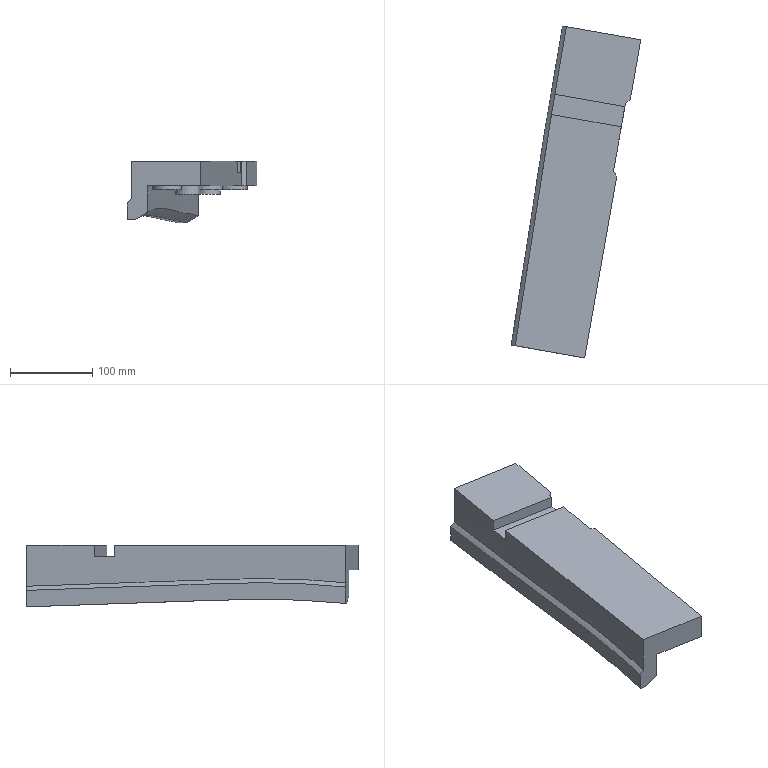Part | NX | features solid 2 | 1 solid | 31 faces | box 157.465 x 403.232 x 74.874 mm | volume 1367300 mm3 | plane 19 | spline 6 | cylinder 6 | commonest cylinder face diameters 35 x4 30 x2